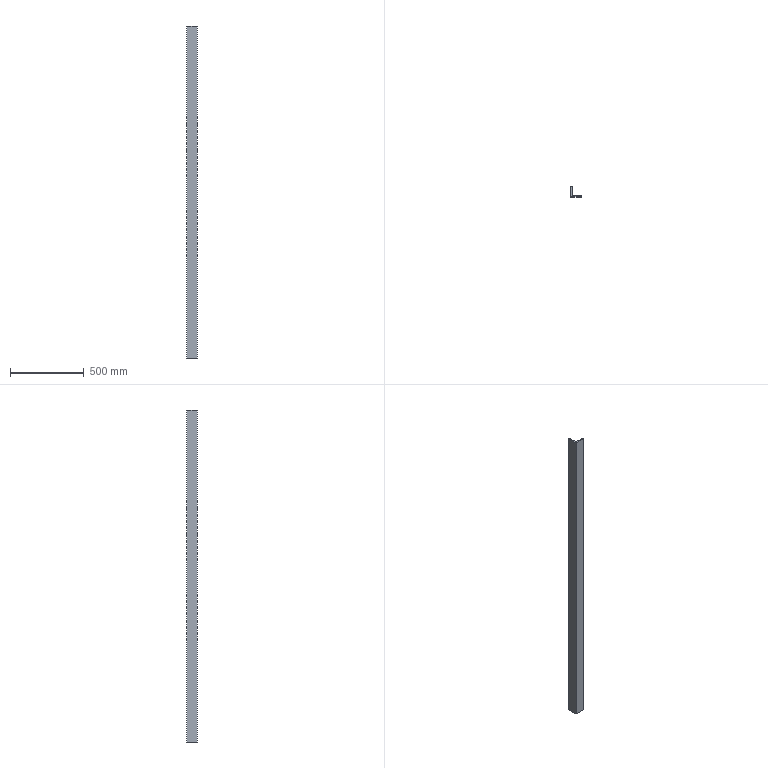Part | SolidWorks | features Extrusion 1 | 1 solid | 11 faces | box 70 x 70 x 2250 mm | volume 2398211 mm3 | plane 8 | cylinder 3 | commonest cylinder face diameters 6 x2 16 x1
STEP:
#1=CARTESIAN_POINT('',(5.,70.,0.));
#2=VERTEX_POINT('',#1);
#3=CARTESIAN_POINT('',(0.,70.,0.));
#4=VERTEX_POINT('',#3);
#5=CARTESIAN_POINT('',(5.,70.,0.));
#6=DIRECTION('',(-1.,0.,0.));
#7=VECTOR('',#6,1000.);
#8=LINE('',#5,#7);
#9=EDGE_CURVE('',#2,#4,#8,.T.);
#10=ORIENTED_EDGE('',*,*,#9,.T.);
#11=CARTESIAN_POINT('',(0.,70.,2250.));
#12=VERTEX_POINT('',#11);
#13=CARTESIAN_POINT('',(0.,70.,2250.));
#14=DIRECTION('',(0.,0.,-1.));
#15=VECTOR('',#14,1000.);
#16=LINE('',#13,#15);
#17=EDGE_CURVE('',#12,#4,#16,.T.);
#18=ORIENTED_EDGE('',*,*,#17,.F.);
#19=CARTESIAN_POINT('',(5.,70.,2250.));
#20=VERTEX_POINT('',#19);
#21=CARTESIAN_POINT('',(5.,70.,2250.));
#22=DIRECTION('',(-1.,0.,0.));
#23=VECTOR('',#22,1000.);
#24=LINE('',#21,#23);
#25=EDGE_CURVE('',#20,#12,#24,.T.);
#26=ORIENTED_EDGE('',*,*,#25,.F.);
#27=CARTESIAN_POINT('',(5.,70.,2250.));
#28=DIRECTION('',(0.,0.,-1.));
#29=VECTOR('',#28,1000.);
#30=LINE('',#27,#29);
#31=EDGE_CURVE('',#20,#2,#30,.T.);
#32=ORIENTED_EDGE('',*,*,#31,.T.);
#33=EDGE_LOOP('',(#10,#18,#26,#32));
#34=FACE_OUTER_BOUND('',#33,.T.);
#35=CARTESIAN_POINT('',(5.,70.,2250.));
#36=DIRECTION('',(0.,-1.,0.));
#37=DIRECTION('',(0.,0.,-1.));
#38=AXIS2_PLACEMENT_3D('',#35,#36,#37);
#39=PLANE('',#38);
#40=ADVANCED_FACE('',(#34),#39,.F.);
#41=CARTESIAN_POINT('',(0.,0.,0.));
#42=VERTEX_POINT('',#41);
#43=CARTESIAN_POINT('',(0.,70.,0.));
#44=DIRECTION('',(0.,-1.,0.));
#45=VECTOR('',#44,1000.);
#46=LINE('',#43,#45);
#47=EDGE_CURVE('',#4,#42,#46,.T.);
#48=ORIENTED_EDGE('',*,*,#47,.T.);
#49=CARTESIAN_POINT('',(0.,0.,2250.));
#50=VERTEX_POINT('',#49);
#51=CARTESIAN_POINT('',(0.,0.,2250.));
#52=DIRECTION('',(0.,0.,-1.));
#53=VECTOR('',#52,1000.);
#54=LINE('',#51,#53);
#55=EDGE_CURVE('',#50,#42,#54,.T.);
#56=ORIENTED_EDGE('',*,*,#55,.F.);
#57=CARTESIAN_POINT('',(0.,70.,2250.));
#58=DIRECTION('',(0.,-1.,0.));
#59=VECTOR('',#58,1000.);
#60=LINE('',#57,#59);
#61=EDGE_CURVE('',#12,#50,#60,.T.);
#62=ORIENTED_EDGE('',*,*,#61,.F.);
#63=ORIENTED_EDGE('',*,*,#17,.T.);
#64=EDGE_LOOP('',(#48,#56,#62,#63));
#65=FACE_OUTER_BOUND('',#64,.T.);
#66=CARTESIAN_POINT('',(0.,70.,2250.));
#67=DIRECTION('',(1.,0.,0.));
#68=DIRECTION('',(0.,0.,-1.));
#69=AXIS2_PLACEMENT_3D('',#66,#67,#68);
#70=PLANE('',#69);
#71=ADVANCED_FACE('',(#65),#70,.F.);
#72=CARTESIAN_POINT('',(70.,0.,0.));
#73=VERTEX_POINT('',#72);
#74=CARTESIAN_POINT('',(0.,0.,0.));
#75=DIRECTION('',(1.,0.,0.));
#76=VECTOR('',#75,1000.);
#77=LINE('',#74,#76);
#78=EDGE_CURVE('',#42,#73,#77,.T.);
#79=ORIENTED_EDGE('',*,*,#78,.T.);
#80=CARTESIAN_POINT('',(70.,0.,2250.));
#81=VERTEX_POINT('',#80);
#82=CARTESIAN_POINT('',(70.,0.,2250.));
#83=DIRECTION('',(0.,0.,-1.));
#84=VECTOR('',#83,1000.);
#85=LINE('',#82,#84);
#86=EDGE_CURVE('',#81,#73,#85,.T.);
#87=ORIENTED_EDGE('',*,*,#86,.F.);
#88=CARTESIAN_POINT('',(0.,0.,2250.));
#89=DIRECTION('',(1.,0.,0.));
#90=VECTOR('',#89,1000.);
#91=LINE('',#88,#90);
#92=EDGE_CURVE('',#50,#81,#91,.T.);
#93=ORIENTED_EDGE('',*,*,#92,.F.);
#94=ORIENTED_EDGE('',*,*,#55,.T.);
#95=EDGE_LOOP('',(#79,#87,#93,#94));
#96=FACE_OUTER_BOUND('',#95,.T.);
#97=CARTESIAN_POINT('',(0.,0.,2250.));
#98=DIRECTION('',(0.,1.,0.));
#99=DIRECTION('',(0.,0.,1.));
#100=AXIS2_PLACEMENT_3D('',#97,#98,#99);
#101=PLANE('',#100);
#102=ADVANCED_FACE('',(#96),#101,.F.);
#103=CARTESIAN_POINT('',(70.,5.,0.));
#104=VERTEX_POINT('',#103);
#105=CARTESIAN_POINT('',(70.,0.,0.));
#106=DIRECTION('',(0.,1.,0.));
#107=VECTOR('',#106,1000.);
#108=LINE('',#105,#107);
#109=EDGE_CURVE('',#73,#104,#108,.T.);
#110=ORIENTED_EDGE('',*,*,#109,.T.);
#111=CARTESIAN_POINT('',(70.,5.,2250.));
#112=VERTEX_POINT('',#111);
#113=CARTESIAN_POINT('',(70.,5.,2250.));
#114=DIRECTION('',(0.,0.,-1.));
#115=VECTOR('',#114,1000.);
#116=LINE('',#113,#115);
#117=EDGE_CURVE('',#112,#104,#116,.T.);
#118=ORIENTED_EDGE('',*,*,#117,.F.);
#119=CARTESIAN_POINT('',(70.,0.,2250.));
#120=DIRECTION('',(0.,1.,0.));
#121=VECTOR('',#120,1000.);
#122=LINE('',#119,#121);
#123=EDGE_CURVE('',#81,#112,#122,.T.);
#124=ORIENTED_EDGE('',*,*,#123,.F.);
#125=ORIENTED_EDGE('',*,*,#86,.T.);
#126=EDGE_LOOP('',(#110,#118,#124,#125));
#127=FACE_OUTER_BOUND('',#126,.T.);
#128=CARTESIAN_POINT('',(70.,0.,2250.));
#129=DIRECTION('',(-1.,0.,0.));
#130=DIRECTION('',(0.,0.,1.));
#131=AXIS2_PLACEMENT_3D('',#128,#129,#130);
#132=PLANE('',#131);
#133=ADVANCED_FACE('',(#127),#132,.F.);
#134=CARTESIAN_POINT('',(67.,8.,0.));
#135=VERTEX_POINT('',#134);
#136=CARTESIAN_POINT('',(67.,5.,0.));
#137=DIRECTION('',(0.,0.,1.));
#138=DIRECTION('',(1.,0.,0.));
#139=AXIS2_PLACEMENT_3D('',#136,#137,#138);
#140=CIRCLE('',#139,3.);
#141=EDGE_CURVE('',#104,#135,#140,.T.);
#142=ORIENTED_EDGE('',*,*,#141,.T.);
#143=CARTESIAN_POINT('',(67.,8.,2250.));
#144=VERTEX_POINT('',#143);
#145=CARTESIAN_POINT('',(67.,8.,2250.));
#146=DIRECTION('',(0.,0.,-1.));
#147=VECTOR('',#146,1000.);
#148=LINE('',#145,#147);
#149=EDGE_CURVE('',#144,#135,#148,.T.);
#150=ORIENTED_EDGE('',*,*,#149,.F.);
#151=CARTESIAN_POINT('',(67.,5.,2250.));
#152=DIRECTION('',(0.,0.,1.));
#153=DIRECTION('',(1.,0.,0.));
#154=AXIS2_PLACEMENT_3D('',#151,#152,#153);
#155=CIRCLE('',#154,3.);
#156=EDGE_CURVE('',#112,#144,#155,.T.);
#157=ORIENTED_EDGE('',*,*,#156,.F.);
#158=ORIENTED_EDGE('',*,*,#117,.T.);
#159=EDGE_LOOP('',(#142,#150,#157,#158));
#160=FACE_OUTER_BOUND('',#159,.T.);
#161=CARTESIAN_POINT('',(67.,5.,2250.));
#162=DIRECTION('',(0.,0.,-1.));
#163=DIRECTION('',(-1.,0.,0.));
#164=AXIS2_PLACEMENT_3D('',#161,#162,#163);
#165=CYLINDRICAL_SURFACE('',#164,3.);
#166=ADVANCED_FACE('',(#160),#165,.T.);
#167=CARTESIAN_POINT('',(16.,8.,0.));
#168=VERTEX_POINT('',#167);
#169=CARTESIAN_POINT('',(67.,8.,0.));
#170=DIRECTION('',(-1.,0.,0.));
#171=VECTOR('',#170,1000.);
#172=LINE('',#169,#171);
#173=EDGE_CURVE('',#135,#168,#172,.T.);
#174=ORIENTED_EDGE('',*,*,#173,.T.);
#175=CARTESIAN_POINT('',(16.,8.,2250.));
#176=VERTEX_POINT('',#175);
#177=CARTESIAN_POINT('',(16.,8.,2250.));
#178=DIRECTION('',(0.,0.,-1.));
#179=VECTOR('',#178,1000.);
#180=LINE('',#177,#179);
#181=EDGE_CURVE('',#176,#168,#180,.T.);
#182=ORIENTED_EDGE('',*,*,#181,.F.);
#183=CARTESIAN_POINT('',(67.,8.,2250.));
#184=DIRECTION('',(-1.,0.,0.));
#185=VECTOR('',#184,1000.);
#186=LINE('',#183,#185);
#187=EDGE_CURVE('',#144,#176,#186,.T.);
#188=ORIENTED_EDGE('',*,*,#187,.F.);
#189=ORIENTED_EDGE('',*,*,#149,.T.);
#190=EDGE_LOOP('',(#174,#182,#188,#189));
#191=FACE_OUTER_BOUND('',#190,.T.);
#192=CARTESIAN_POINT('',(67.,8.,2250.));
#193=DIRECTION('',(0.,-1.,0.));
#194=DIRECTION('',(1.,0.,0.));
#195=AXIS2_PLACEMENT_3D('',#192,#193,#194);
#196=PLANE('',#195);
#197=ADVANCED_FACE('',(#191),#196,.F.);
#198=CARTESIAN_POINT('',(8.,16.,0.));
#199=VERTEX_POINT('',#198);
#200=CARTESIAN_POINT('',(16.,16.,0.));
#201=DIRECTION('',(0.,0.,-1.));
#202=DIRECTION('',(-1.,0.,0.));
#203=AXIS2_PLACEMENT_3D('',#200,#201,#202);
#204=CIRCLE('',#203,8.);
#205=EDGE_CURVE('',#168,#199,#204,.T.);
#206=ORIENTED_EDGE('',*,*,#205,.T.);
#207=CARTESIAN_POINT('',(8.,16.,2250.));
#208=VERTEX_POINT('',#207);
#209=CARTESIAN_POINT('',(8.,16.,2250.));
#210=DIRECTION('',(0.,0.,-1.));
#211=VECTOR('',#210,1000.);
#212=LINE('',#209,#211);
#213=EDGE_CURVE('',#208,#199,#212,.T.);
#214=ORIENTED_EDGE('',*,*,#213,.F.);
#215=CARTESIAN_POINT('',(16.,16.,2250.));
#216=DIRECTION('',(0.,0.,-1.));
#217=DIRECTION('',(-1.,0.,0.));
#218=AXIS2_PLACEMENT_3D('',#215,#216,#217);
#219=CIRCLE('',#218,8.);
#220=EDGE_CURVE('',#176,#208,#219,.T.);
#221=ORIENTED_EDGE('',*,*,#220,.F.);
#222=ORIENTED_EDGE('',*,*,#181,.T.);
#223=EDGE_LOOP('',(#206,#214,#221,#222));
#224=FACE_OUTER_BOUND('',#223,.T.);
#225=CARTESIAN_POINT('',(16.,16.,2250.));
#226=DIRECTION('',(0.,0.,-1.));
#227=DIRECTION('',(-1.,0.,0.));
#228=AXIS2_PLACEMENT_3D('',#225,#226,#227);
#229=CYLINDRICAL_SURFACE('',#228,8.);
#230=ADVANCED_FACE('',(#224),#229,.F.);
#231=CARTESIAN_POINT('',(8.,67.,0.));
#232=VERTEX_POINT('',#231);
#233=CARTESIAN_POINT('',(8.,16.,0.));
#234=DIRECTION('',(0.,1.,0.));
#235=VECTOR('',#234,1000.);
#236=LINE('',#233,#235);
#237=EDGE_CURVE('',#199,#232,#236,.T.);
#238=ORIENTED_EDGE('',*,*,#237,.T.);
#239=CARTESIAN_POINT('',(8.,67.,2250.));
#240=VERTEX_POINT('',#239);
#241=CARTESIAN_POINT('',(8.,67.,2250.));
#242=DIRECTION('',(0.,0.,-1.));
#243=VECTOR('',#242,1000.);
#244=LINE('',#241,#243);
#245=EDGE_CURVE('',#240,#232,#244,.T.);
#246=ORIENTED_EDGE('',*,*,#245,.F.);
#247=CARTESIAN_POINT('',(8.,16.,2250.));
#248=DIRECTION('',(0.,1.,0.));
#249=VECTOR('',#248,1000.);
#250=LINE('',#247,#249);
#251=EDGE_CURVE('',#208,#240,#250,.T.);
#252=ORIENTED_EDGE('',*,*,#251,.F.);
#253=ORIENTED_EDGE('',*,*,#213,.T.);
#254=EDGE_LOOP('',(#238,#246,#252,#253));
#255=FACE_OUTER_BOUND('',#254,.T.);
#256=CARTESIAN_POINT('',(8.,16.,2250.));
#257=DIRECTION('',(-1.,0.,0.));
#258=DIRECTION('',(0.,-1.,0.));
#259=AXIS2_PLACEMENT_3D('',#256,#257,#258);
#260=PLANE('',#259);
#261=ADVANCED_FACE('',(#255),#260,.F.);
#262=CARTESIAN_POINT('',(5.,67.,0.));
#263=DIRECTION('',(0.,0.,1.));
#264=DIRECTION('',(1.,0.,0.));
#265=AXIS2_PLACEMENT_3D('',#262,#263,#264);
#266=CIRCLE('',#265,3.);
#267=EDGE_CURVE('',#232,#2,#266,.T.);
#268=ORIENTED_EDGE('',*,*,#267,.T.);
#269=ORIENTED_EDGE('',*,*,#31,.F.);
#270=CARTESIAN_POINT('',(5.,67.,2250.));
#271=DIRECTION('',(0.,0.,1.));
#272=DIRECTION('',(1.,0.,0.));
#273=AXIS2_PLACEMENT_3D('',#270,#271,#272);
#274=CIRCLE('',#273,3.);
#275=EDGE_CURVE('',#240,#20,#274,.T.);
#276=ORIENTED_EDGE('',*,*,#275,.F.);
#277=ORIENTED_EDGE('',*,*,#245,.T.);
#278=EDGE_LOOP('',(#268,#269,#276,#277));
#279=FACE_OUTER_BOUND('',#278,.T.);
#280=CARTESIAN_POINT('',(5.,67.,2250.));
#281=DIRECTION('',(0.,0.,-1.));
#282=DIRECTION('',(-1.,0.,0.));
#283=AXIS2_PLACEMENT_3D('',#280,#281,#282);
#284=CYLINDRICAL_SURFACE('',#283,3.);
#285=ADVANCED_FACE('',(#279),#284,.T.);
#286=ORIENTED_EDGE('',*,*,#25,.T.);
#287=ORIENTED_EDGE('',*,*,#61,.T.);
#288=ORIENTED_EDGE('',*,*,#92,.T.);
#289=ORIENTED_EDGE('',*,*,#123,.T.);
#290=ORIENTED_EDGE('',*,*,#156,.T.);
#291=ORIENTED_EDGE('',*,*,#187,.T.);
#292=ORIENTED_EDGE('',*,*,#220,.T.);
#293=ORIENTED_EDGE('',*,*,#251,.T.);
#294=ORIENTED_EDGE('',*,*,#275,.T.);
#295=EDGE_LOOP('',(#286,#287,#288,#289,#290,#291,#292,#293,#294));
#296=FACE_OUTER_BOUND('',#295,.T.);
#297=CARTESIAN_POINT('',(67.,5.,2250.));
#298=DIRECTION('',(0.,0.,1.));
#299=DIRECTION('',(1.,0.,0.));
#300=AXIS2_PLACEMENT_3D('',#297,#298,#299);
#301=PLANE('',#300);
#302=ADVANCED_FACE('',(#296),#301,.T.);
#303=ORIENTED_EDGE('',*,*,#9,.F.);
#304=ORIENTED_EDGE('',*,*,#267,.F.);
#305=ORIENTED_EDGE('',*,*,#237,.F.);
#306=ORIENTED_EDGE('',*,*,#205,.F.);
#307=ORIENTED_EDGE('',*,*,#173,.F.);
#308=ORIENTED_EDGE('',*,*,#141,.F.);
#309=ORIENTED_EDGE('',*,*,#109,.F.);
#310=ORIENTED_EDGE('',*,*,#78,.F.);
#311=ORIENTED_EDGE('',*,*,#47,.F.);
#312=EDGE_LOOP('',(#303,#304,#305,#306,#307,#308,#309,#310,#311));
#313=FACE_OUTER_BOUND('',#312,.T.);
#314=CARTESIAN_POINT('',(67.,5.,0.));
#315=DIRECTION('',(0.,0.,1.));
#316=DIRECTION('',(1.,0.,0.));
#317=AXIS2_PLACEMENT_3D('',#314,#315,#316);
#318=PLANE('',#317);
#319=ADVANCED_FACE('',(#313),#318,.F.);
#320=CLOSED_SHELL('',(#40,#71,#102,#133,#166,#197,#230,#261,#285,#302,#319));
#321=MANIFOLD_SOLID_BREP('',#320);
#322=CARTESIAN_POINT('',(0.,0.,0.));
#323=DIRECTION('',(0.,0.,1.));
#324=DIRECTION('',(1.,0.,0.));
#325=AXIS2_PLACEMENT_3D('',#322,#323,#324);
#326=(LENGTH_UNIT()NAMED_UNIT(*)SI_UNIT(.MILLI.,.METRE.));
#327=UNCERTAINTY_MEASURE_WITH_UNIT(LENGTH_MEASURE(0.00001),#326,'','');
#328=(NAMED_UNIT(*)PLANE_ANGLE_UNIT()SI_UNIT($,.RADIAN.));
#329=(NAMED_UNIT(*)SI_UNIT($,.STERADIAN.)SOLID_ANGLE_UNIT());
#330=(GEOMETRIC_REPRESENTATION_CONTEXT(3)GLOBAL_UNCERTAINTY_ASSIGNED_CONTEXT((#327))GLOBAL_UNIT_ASSIGNED_CONTEXT((#326,#328,#329))REPRESENTATION_CONTEXT('',''));
#331=ADVANCED_BREP_SHAPE_REPRESENTATION('',(#321,#325),#330);